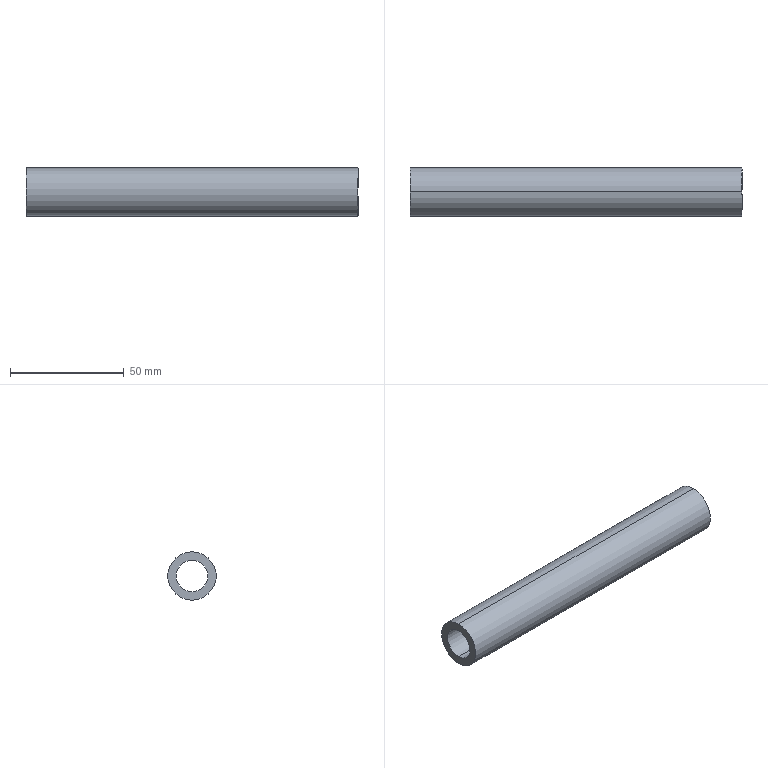Part | SolidWorks | features BaseBody 1 | 1 solid | 6 faces | box 145.797 x 21.234 x 21.234 mm | volume 29608 mm3 | cylinder 4 | plane 2 | commonest cylinder face diameters 13.868 x2 21.234 x2
STEP:
#1=CARTESIAN_POINT('',(152.408,6.088,-6.934));
#2=VERTEX_POINT('',#1);
#3=CARTESIAN_POINT('',(152.408,6.088,6.934));
#4=VERTEX_POINT('',#3);
#5=CARTESIAN_POINT('',(152.408,6.088,0.));
#6=DIRECTION('',(1.,0.,0.));
#7=DIRECTION('',(0.,0.,-1.));
#8=AXIS2_PLACEMENT_3D('',#5,#6,#7);
#9=CIRCLE('',#8,6.934);
#10=EDGE_CURVE('',#2,#4,#9,.T.);
#11=ORIENTED_EDGE('',*,*,#10,.F.);
#12=CARTESIAN_POINT('',(152.408,6.088,0.));
#13=DIRECTION('',(1.,0.,0.));
#14=DIRECTION('',(0.,0.,1.));
#15=AXIS2_PLACEMENT_3D('',#12,#13,#14);
#16=CIRCLE('',#15,6.934);
#17=EDGE_CURVE('',#4,#2,#16,.T.);
#18=ORIENTED_EDGE('',*,*,#17,.F.);
#19=EDGE_LOOP('',(#11,#18));
#20=FACE_BOUND('',#19,.T.);
#21=CARTESIAN_POINT('',(152.408,6.088,-10.617));
#22=VERTEX_POINT('',#21);
#23=CARTESIAN_POINT('',(152.408,6.088,10.617));
#24=VERTEX_POINT('',#23);
#25=CARTESIAN_POINT('',(152.408,6.088,0.));
#26=DIRECTION('',(-1.,0.,0.));
#27=DIRECTION('',(0.,0.,-1.));
#28=AXIS2_PLACEMENT_3D('',#25,#26,#27);
#29=CIRCLE('',#28,10.617);
#30=EDGE_CURVE('',#22,#24,#29,.T.);
#31=ORIENTED_EDGE('',*,*,#30,.F.);
#32=CARTESIAN_POINT('',(152.408,6.088,0.));
#33=DIRECTION('',(-1.,0.,0.));
#34=DIRECTION('',(0.,0.,1.));
#35=AXIS2_PLACEMENT_3D('',#32,#33,#34);
#36=CIRCLE('',#35,10.617);
#37=EDGE_CURVE('',#24,#22,#36,.T.);
#38=ORIENTED_EDGE('',*,*,#37,.F.);
#39=EDGE_LOOP('',(#31,#38));
#40=FACE_OUTER_BOUND('',#39,.T.);
#41=CARTESIAN_POINT('',(152.408,6.088,0.));
#42=DIRECTION('',(1.,0.,0.));
#43=DIRECTION('',(0.,1.,0.));
#44=AXIS2_PLACEMENT_3D('',#41,#42,#43);
#45=PLANE('',#44);
#46=ADVANCED_FACE('',(#20,#40),#45,.T.);
#47=CARTESIAN_POINT('',(6.612,6.088,-6.934));
#48=VERTEX_POINT('',#47);
#49=CARTESIAN_POINT('',(6.612,6.088,6.934));
#50=VERTEX_POINT('',#49);
#51=CARTESIAN_POINT('',(6.612,6.088,0.));
#52=DIRECTION('',(-1.,0.,0.));
#53=DIRECTION('',(0.,0.,-1.));
#54=AXIS2_PLACEMENT_3D('',#51,#52,#53);
#55=CIRCLE('',#54,6.934);
#56=EDGE_CURVE('',#48,#50,#55,.T.);
#57=ORIENTED_EDGE('',*,*,#56,.F.);
#58=CARTESIAN_POINT('',(6.612,6.088,0.));
#59=DIRECTION('',(-1.,0.,0.));
#60=DIRECTION('',(0.,0.,1.));
#61=AXIS2_PLACEMENT_3D('',#58,#59,#60);
#62=CIRCLE('',#61,6.934);
#63=EDGE_CURVE('',#50,#48,#62,.T.);
#64=ORIENTED_EDGE('',*,*,#63,.F.);
#65=EDGE_LOOP('',(#57,#64));
#66=FACE_BOUND('',#65,.T.);
#67=CARTESIAN_POINT('',(6.612,6.088,-10.617));
#68=VERTEX_POINT('',#67);
#69=CARTESIAN_POINT('',(6.612,6.088,10.617));
#70=VERTEX_POINT('',#69);
#71=CARTESIAN_POINT('',(6.612,6.088,0.));
#72=DIRECTION('',(1.,0.,0.));
#73=DIRECTION('',(0.,0.,-1.));
#74=AXIS2_PLACEMENT_3D('',#71,#72,#73);
#75=CIRCLE('',#74,10.617);
#76=EDGE_CURVE('',#68,#70,#75,.T.);
#77=ORIENTED_EDGE('',*,*,#76,.F.);
#78=CARTESIAN_POINT('',(6.612,6.088,0.));
#79=DIRECTION('',(1.,0.,0.));
#80=DIRECTION('',(0.,0.,1.));
#81=AXIS2_PLACEMENT_3D('',#78,#79,#80);
#82=CIRCLE('',#81,10.617);
#83=EDGE_CURVE('',#70,#68,#82,.T.);
#84=ORIENTED_EDGE('',*,*,#83,.F.);
#85=EDGE_LOOP('',(#77,#84));
#86=FACE_OUTER_BOUND('',#85,.T.);
#87=CARTESIAN_POINT('',(6.612,6.088,0.));
#88=DIRECTION('',(-1.,0.,0.));
#89=DIRECTION('',(0.,0.,1.));
#90=AXIS2_PLACEMENT_3D('',#87,#88,#89);
#91=PLANE('',#90);
#92=ADVANCED_FACE('',(#66,#86),#91,.T.);
#93=ORIENTED_EDGE('',*,*,#37,.T.);
#94=CARTESIAN_POINT('',(6.612,6.088,-10.617));
#95=DIRECTION('',(1.,0.,0.));
#96=VECTOR('',#95,1000.);
#97=LINE('',#94,#96);
#98=EDGE_CURVE('',#68,#22,#97,.T.);
#99=ORIENTED_EDGE('',*,*,#98,.F.);
#100=ORIENTED_EDGE('',*,*,#76,.T.);
#101=CARTESIAN_POINT('',(152.408,6.088,10.617));
#102=DIRECTION('',(-1.,0.,0.));
#103=VECTOR('',#102,1000.);
#104=LINE('',#101,#103);
#105=EDGE_CURVE('',#24,#70,#104,.T.);
#106=ORIENTED_EDGE('',*,*,#105,.F.);
#107=EDGE_LOOP('',(#93,#99,#100,#106));
#108=FACE_OUTER_BOUND('',#107,.T.);
#109=CARTESIAN_POINT('',(6.612,6.088,0.));
#110=DIRECTION('',(1.,0.,0.));
#111=DIRECTION('',(0.,0.,-1.));
#112=AXIS2_PLACEMENT_3D('',#109,#110,#111);
#113=CYLINDRICAL_SURFACE('',#112,10.617);
#114=ADVANCED_FACE('',(#108),#113,.T.);
#115=ORIENTED_EDGE('',*,*,#105,.T.);
#116=ORIENTED_EDGE('',*,*,#83,.T.);
#117=ORIENTED_EDGE('',*,*,#98,.T.);
#118=ORIENTED_EDGE('',*,*,#30,.T.);
#119=EDGE_LOOP('',(#115,#116,#117,#118));
#120=FACE_OUTER_BOUND('',#119,.T.);
#121=CARTESIAN_POINT('',(6.612,6.088,0.));
#122=DIRECTION('',(1.,0.,0.));
#123=DIRECTION('',(0.,0.,-1.));
#124=AXIS2_PLACEMENT_3D('',#121,#122,#123);
#125=CYLINDRICAL_SURFACE('',#124,10.617);
#126=ADVANCED_FACE('',(#120),#125,.T.);
#127=ORIENTED_EDGE('',*,*,#17,.T.);
#128=CARTESIAN_POINT('',(6.612,6.088,-6.934));
#129=DIRECTION('',(1.,0.,0.));
#130=VECTOR('',#129,1000.);
#131=LINE('',#128,#130);
#132=EDGE_CURVE('',#48,#2,#131,.T.);
#133=ORIENTED_EDGE('',*,*,#132,.F.);
#134=ORIENTED_EDGE('',*,*,#56,.T.);
#135=CARTESIAN_POINT('',(152.408,6.088,6.934));
#136=DIRECTION('',(-1.,0.,0.));
#137=VECTOR('',#136,1000.);
#138=LINE('',#135,#137);
#139=EDGE_CURVE('',#4,#50,#138,.T.);
#140=ORIENTED_EDGE('',*,*,#139,.F.);
#141=EDGE_LOOP('',(#127,#133,#134,#140));
#142=FACE_OUTER_BOUND('',#141,.T.);
#143=CARTESIAN_POINT('',(6.612,6.088,0.));
#144=DIRECTION('',(1.,0.,0.));
#145=DIRECTION('',(0.,0.,-1.));
#146=AXIS2_PLACEMENT_3D('',#143,#144,#145);
#147=CYLINDRICAL_SURFACE('',#146,6.934);
#148=ADVANCED_FACE('',(#142),#147,.F.);
#149=ORIENTED_EDGE('',*,*,#139,.T.);
#150=ORIENTED_EDGE('',*,*,#63,.T.);
#151=ORIENTED_EDGE('',*,*,#132,.T.);
#152=ORIENTED_EDGE('',*,*,#10,.T.);
#153=EDGE_LOOP('',(#149,#150,#151,#152));
#154=FACE_OUTER_BOUND('',#153,.T.);
#155=CARTESIAN_POINT('',(6.612,6.088,0.));
#156=DIRECTION('',(1.,0.,0.));
#157=DIRECTION('',(0.,0.,-1.));
#158=AXIS2_PLACEMENT_3D('',#155,#156,#157);
#159=CYLINDRICAL_SURFACE('',#158,6.934);
#160=ADVANCED_FACE('',(#154),#159,.F.);
#161=CLOSED_SHELL('',(#46,#92,#114,#126,#148,#160));
#162=MANIFOLD_SOLID_BREP('',#161);
#163=CARTESIAN_POINT('',(0.,0.,0.));
#164=DIRECTION('',(0.,0.,1.));
#165=DIRECTION('',(1.,0.,0.));
#166=AXIS2_PLACEMENT_3D('',#163,#164,#165);
#167=(LENGTH_UNIT()NAMED_UNIT(*)SI_UNIT(.MILLI.,.METRE.));
#168=UNCERTAINTY_MEASURE_WITH_UNIT(LENGTH_MEASURE(0.00001),#167,'','');
#169=(NAMED_UNIT(*)PLANE_ANGLE_UNIT()SI_UNIT($,.RADIAN.));
#170=(NAMED_UNIT(*)SI_UNIT($,.STERADIAN.)SOLID_ANGLE_UNIT());
#171=(GEOMETRIC_REPRESENTATION_CONTEXT(3)GLOBAL_UNCERTAINTY_ASSIGNED_CONTEXT((#168))GLOBAL_UNIT_ASSIGNED_CONTEXT((#167,#169,#170))REPRESENTATION_CONTEXT('',''));
#172=ADVANCED_BREP_SHAPE_REPRESENTATION('',(#162,#166),#171);